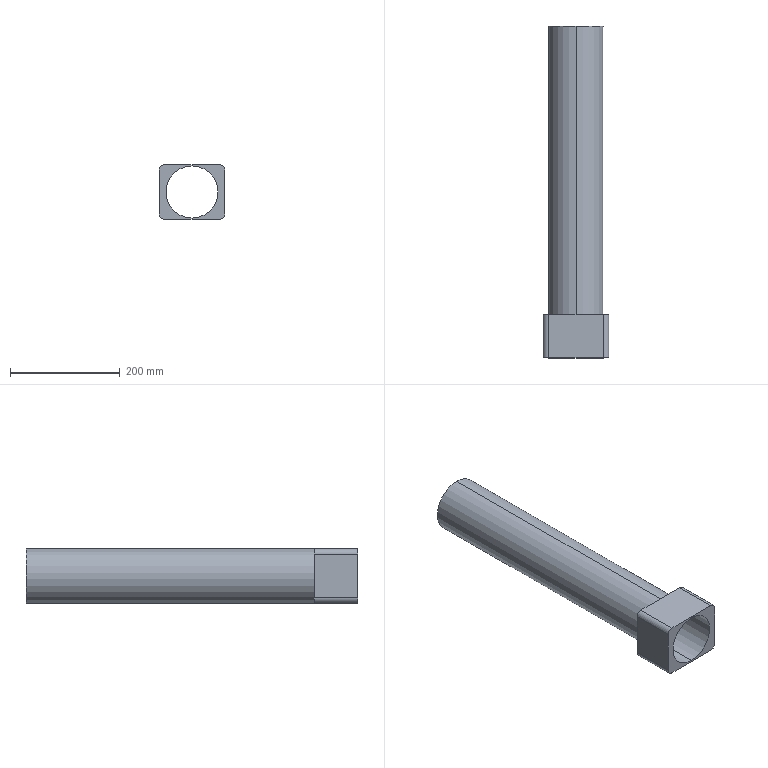Part | STEP file | Drain pipe 1 | 1 solid | 16 faces | box 120 x 605 x 100 mm | volume 788101 mm3 | cylinder 8 | plane 8 | commonest cylinder face diameters 20 x4 95 x2 100 x2
STEP:
#1=CARTESIAN_POINT('',(0.,0.,0.));
#2=DIRECTION('',(0.,0.,1.));
#3=DIRECTION('',(1.,0.,0.));
#4=AXIS2_PLACEMENT_3D('',#1,#2,#3);
#5=CARTESIAN_POINT('',(60.,605.,100.));
#6=VERTEX_POINT('',#5);
#7=CARTESIAN_POINT('',(60.,605.,0.));
#8=VERTEX_POINT('',#7);
#9=CARTESIAN_POINT('',(60.,605.,50.));
#10=DIRECTION('',(0.,1.,0.));
#11=DIRECTION('',(0.,0.,1.));
#12=AXIS2_PLACEMENT_3D('',#9,#10,#11);
#13=CIRCLE('',#12,50.);
#14=CARTESIAN_POINT('',(60.,605.,50.));
#15=DIRECTION('',(0.,-1.,0.));
#16=DIRECTION('',(0.,0.,-1.));
#17=AXIS2_PLACEMENT_3D('',#14,#15,#16);
#18=CYLINDRICAL_SURFACE('',#17,50.);
#19=CARTESIAN_POINT('',(3.142,0.));
#20=DIRECTION('',(-1.,0.));
#21=VECTOR('',#20,1.);
#22=LINE('',#19,#21);
#23=(GEOMETRIC_REPRESENTATION_CONTEXT(2)PARAMETRIC_REPRESENTATION_CONTEXT()REPRESENTATION_CONTEXT('',''));
#24=DEFINITIONAL_REPRESENTATION('',(#22),#23);
#25=PCURVE('',#18,#24);
#26=CARTESIAN_POINT('',(60.,605.,50.));
#27=DIRECTION('',(0.,1.,0.));
#28=DIRECTION('',(0.,0.,1.));
#29=AXIS2_PLACEMENT_3D('',#26,#27,#28);
#30=PLANE('',#29);
#31=CARTESIAN_POINT('',(0.,0.));
#32=DIRECTION('',(1.,0.));
#33=AXIS2_PLACEMENT_2D('',#31,#32);
#34=CIRCLE('',#33,50.);
#35=(GEOMETRIC_REPRESENTATION_CONTEXT(2)PARAMETRIC_REPRESENTATION_CONTEXT()REPRESENTATION_CONTEXT('',''));
#36=DEFINITIONAL_REPRESENTATION('',(#34),#35);
#37=PCURVE('',#30,#36);
#38=SURFACE_CURVE('',#13,(#25,#37),.PCURVE_S1.);
#39=EDGE_CURVE('',#6,#8,#38,.T.);
#40=ORIENTED_EDGE('',*,*,#39,.F.);
#41=CARTESIAN_POINT('',(60.,80.,100.));
#42=VERTEX_POINT('',#41);
#43=CARTESIAN_POINT('',(60.,605.,100.));
#44=DIRECTION('',(0.,-1.,0.));
#45=VECTOR('',#44,1.);
#46=LINE('',#43,#45);
#47=CARTESIAN_POINT('',(3.142,0.));
#48=DIRECTION('',(0.,1.));
#49=VECTOR('',#48,1.);
#50=LINE('',#47,#49);
#51=(GEOMETRIC_REPRESENTATION_CONTEXT(2)PARAMETRIC_REPRESENTATION_CONTEXT()REPRESENTATION_CONTEXT('',''));
#52=DEFINITIONAL_REPRESENTATION('',(#50),#51);
#53=PCURVE('',#18,#52);
#54=CARTESIAN_POINT('',(60.,605.,50.));
#55=DIRECTION('',(0.,-1.,0.));
#56=DIRECTION('',(0.,0.,-1.));
#57=AXIS2_PLACEMENT_3D('',#54,#55,#56);
#58=CYLINDRICAL_SURFACE('',#57,50.);
#59=CARTESIAN_POINT('',(3.142,0.));
#60=DIRECTION('',(0.,1.));
#61=VECTOR('',#60,1.);
#62=LINE('',#59,#61);
#63=(GEOMETRIC_REPRESENTATION_CONTEXT(2)PARAMETRIC_REPRESENTATION_CONTEXT()REPRESENTATION_CONTEXT('',''));
#64=DEFINITIONAL_REPRESENTATION('',(#62),#63);
#65=PCURVE('',#58,#64);
#66=SURFACE_CURVE('',#46,(#53,#65),.PCURVE_S1.);
#67=EDGE_CURVE('',#6,#42,#66,.T.);
#68=ORIENTED_EDGE('',*,*,#67,.T.);
#69=CARTESIAN_POINT('',(60.,80.,0.));
#70=VERTEX_POINT('',#69);
#71=CARTESIAN_POINT('',(60.,80.,50.));
#72=DIRECTION('',(0.,1.,0.));
#73=DIRECTION('',(0.,0.,1.));
#74=AXIS2_PLACEMENT_3D('',#71,#72,#73);
#75=CIRCLE('',#74,50.);
#76=CARTESIAN_POINT('',(3.142,525.));
#77=DIRECTION('',(-1.,0.));
#78=VECTOR('',#77,1.);
#79=LINE('',#76,#78);
#80=(GEOMETRIC_REPRESENTATION_CONTEXT(2)PARAMETRIC_REPRESENTATION_CONTEXT()REPRESENTATION_CONTEXT('',''));
#81=DEFINITIONAL_REPRESENTATION('',(#79),#80);
#82=PCURVE('',#18,#81);
#83=CARTESIAN_POINT('',(0.,80.,100.));
#84=DIRECTION('',(0.,1.,0.));
#85=DIRECTION('',(0.,0.,1.));
#86=AXIS2_PLACEMENT_3D('',#83,#84,#85);
#87=PLANE('',#86);
#88=CARTESIAN_POINT('',(-50.,60.));
#89=DIRECTION('',(1.,0.));
#90=AXIS2_PLACEMENT_2D('',#88,#89);
#91=CIRCLE('',#90,50.);
#92=(GEOMETRIC_REPRESENTATION_CONTEXT(2)PARAMETRIC_REPRESENTATION_CONTEXT()REPRESENTATION_CONTEXT('',''));
#93=DEFINITIONAL_REPRESENTATION('',(#91),#92);
#94=PCURVE('',#87,#93);
#95=SURFACE_CURVE('',#75,(#82,#94),.PCURVE_S1.);
#96=EDGE_CURVE('',#42,#70,#95,.T.);
#97=ORIENTED_EDGE('',*,*,#96,.T.);
#98=CARTESIAN_POINT('',(60.,605.,0.));
#99=DIRECTION('',(0.,-1.,0.));
#100=VECTOR('',#99,1.);
#101=LINE('',#98,#100);
#102=CARTESIAN_POINT('',(0.,0.));
#103=DIRECTION('',(0.,1.));
#104=VECTOR('',#103,1.);
#105=LINE('',#102,#104);
#106=(GEOMETRIC_REPRESENTATION_CONTEXT(2)PARAMETRIC_REPRESENTATION_CONTEXT()REPRESENTATION_CONTEXT('',''));
#107=DEFINITIONAL_REPRESENTATION('',(#105),#106);
#108=PCURVE('',#18,#107);
#109=CARTESIAN_POINT('',(6.283,0.));
#110=DIRECTION('',(0.,1.));
#111=VECTOR('',#110,1.);
#112=LINE('',#109,#111);
#113=(GEOMETRIC_REPRESENTATION_CONTEXT(2)PARAMETRIC_REPRESENTATION_CONTEXT()REPRESENTATION_CONTEXT('',''));
#114=DEFINITIONAL_REPRESENTATION('',(#112),#113);
#115=PCURVE('',#58,#114);
#116=SURFACE_CURVE('',#101,(#108,#115),.PCURVE_S1.);
#117=EDGE_CURVE('',#8,#70,#116,.T.);
#118=ORIENTED_EDGE('',*,*,#117,.F.);
#119=EDGE_LOOP('',(#40,#68,#97,#118));
#120=FACE_BOUND('',#119,.T.);
#121=ADVANCED_FACE('',(#120),#18,.T.);
#122=CARTESIAN_POINT('',(60.,605.,2.5));
#123=VERTEX_POINT('',#122);
#124=CARTESIAN_POINT('',(60.,0.,2.5));
#125=VERTEX_POINT('',#124);
#126=CARTESIAN_POINT('',(60.,605.,2.5));
#127=DIRECTION('',(0.,-1.,0.));
#128=VECTOR('',#127,1.);
#129=LINE('',#126,#128);
#130=CARTESIAN_POINT('',(60.,605.,50.));
#131=DIRECTION('',(0.,-1.,0.));
#132=DIRECTION('',(0.,0.,-1.));
#133=AXIS2_PLACEMENT_3D('',#130,#131,#132);
#134=CYLINDRICAL_SURFACE('',#133,47.5);
#135=CARTESIAN_POINT('',(6.283,0.));
#136=DIRECTION('',(0.,1.));
#137=VECTOR('',#136,1.);
#138=LINE('',#135,#137);
#139=(GEOMETRIC_REPRESENTATION_CONTEXT(2)PARAMETRIC_REPRESENTATION_CONTEXT()REPRESENTATION_CONTEXT('',''));
#140=DEFINITIONAL_REPRESENTATION('',(#138),#139);
#141=PCURVE('',#134,#140);
#142=CARTESIAN_POINT('',(60.,605.,50.));
#143=DIRECTION('',(0.,-1.,0.));
#144=DIRECTION('',(0.,0.,-1.));
#145=AXIS2_PLACEMENT_3D('',#142,#143,#144);
#146=CYLINDRICAL_SURFACE('',#145,47.5);
#147=CARTESIAN_POINT('',(0.,0.));
#148=DIRECTION('',(0.,1.));
#149=VECTOR('',#148,1.);
#150=LINE('',#147,#149);
#151=(GEOMETRIC_REPRESENTATION_CONTEXT(2)PARAMETRIC_REPRESENTATION_CONTEXT()REPRESENTATION_CONTEXT('',''));
#152=DEFINITIONAL_REPRESENTATION('',(#150),#151);
#153=PCURVE('',#146,#152);
#154=SURFACE_CURVE('',#129,(#141,#153),.PCURVE_S1.);
#155=EDGE_CURVE('',#123,#125,#154,.T.);
#156=ORIENTED_EDGE('',*,*,#155,.T.);
#157=CARTESIAN_POINT('',(60.,0.,97.5));
#158=VERTEX_POINT('',#157);
#159=CARTESIAN_POINT('',(60.,0.,50.));
#160=DIRECTION('',(0.,-1.,0.));
#161=DIRECTION('',(0.,0.,-1.));
#162=AXIS2_PLACEMENT_3D('',#159,#160,#161);
#163=CIRCLE('',#162,47.5);
#164=CARTESIAN_POINT('',(0.,605.));
#165=DIRECTION('',(1.,0.));
#166=VECTOR('',#165,1.);
#167=LINE('',#164,#166);
#168=(GEOMETRIC_REPRESENTATION_CONTEXT(2)PARAMETRIC_REPRESENTATION_CONTEXT()REPRESENTATION_CONTEXT('',''));
#169=DEFINITIONAL_REPRESENTATION('',(#167),#168);
#170=PCURVE('',#134,#169);
#171=CARTESIAN_POINT('',(0.,0.,100.));
#172=DIRECTION('',(0.,1.,0.));
#173=DIRECTION('',(0.,0.,1.));
#174=AXIS2_PLACEMENT_3D('',#171,#172,#173);
#175=PLANE('',#174);
#176=CARTESIAN_POINT('',(-97.5,60.));
#177=CARTESIAN_POINT('',(-97.5,142.272));
#178=CARTESIAN_POINT('',(-26.25,101.136));
#179=CARTESIAN_POINT('',(45.,60.));
#180=CARTESIAN_POINT('',(-26.25,18.864));
#181=CARTESIAN_POINT('',(-97.5,-22.272));
#182=CARTESIAN_POINT('',(-97.5,60.));
#183=(BOUNDED_CURVE()B_SPLINE_CURVE(2,(#176,#177,#178,#179,#180,#181,#182),.UNSPECIFIED.,.T.,.F.)B_SPLINE_CURVE_WITH_KNOTS((1,2,2,2,2,1),(-2.094,0.,2.094,4.189,6.283,8.378),.UNSPECIFIED.)CURVE()GEOMETRIC_REPRESENTATION_ITEM()RATIONAL_B_SPLINE_CURVE((1.,0.5,1.,0.5,1.,0.5,1.))REPRESENTATION_ITEM(''));
#184=(GEOMETRIC_REPRESENTATION_CONTEXT(2)PARAMETRIC_REPRESENTATION_CONTEXT()REPRESENTATION_CONTEXT('',''));
#185=DEFINITIONAL_REPRESENTATION('',(#183),#184);
#186=PCURVE('',#175,#185);
#187=SURFACE_CURVE('',#163,(#170,#186),.PCURVE_S1.);
#188=EDGE_CURVE('',#158,#125,#187,.T.);
#189=ORIENTED_EDGE('',*,*,#188,.F.);
#190=CARTESIAN_POINT('',(60.,605.,97.5));
#191=VERTEX_POINT('',#190);
#192=CARTESIAN_POINT('',(60.,605.,97.5));
#193=DIRECTION('',(0.,-1.,0.));
#194=VECTOR('',#193,1.);
#195=LINE('',#192,#194);
#196=CARTESIAN_POINT('',(3.142,0.));
#197=DIRECTION('',(0.,1.));
#198=VECTOR('',#197,1.);
#199=LINE('',#196,#198);
#200=(GEOMETRIC_REPRESENTATION_CONTEXT(2)PARAMETRIC_REPRESENTATION_CONTEXT()REPRESENTATION_CONTEXT('',''));
#201=DEFINITIONAL_REPRESENTATION('',(#199),#200);
#202=PCURVE('',#134,#201);
#203=CARTESIAN_POINT('',(3.142,0.));
#204=DIRECTION('',(0.,1.));
#205=VECTOR('',#204,1.);
#206=LINE('',#203,#205);
#207=(GEOMETRIC_REPRESENTATION_CONTEXT(2)PARAMETRIC_REPRESENTATION_CONTEXT()REPRESENTATION_CONTEXT('',''));
#208=DEFINITIONAL_REPRESENTATION('',(#206),#207);
#209=PCURVE('',#146,#208);
#210=SURFACE_CURVE('',#195,(#202,#209),.PCURVE_S1.);
#211=EDGE_CURVE('',#191,#158,#210,.T.);
#212=ORIENTED_EDGE('',*,*,#211,.F.);
#213=CARTESIAN_POINT('',(60.,605.,50.));
#214=DIRECTION('',(0.,1.,0.));
#215=DIRECTION('',(0.,0.,1.));
#216=AXIS2_PLACEMENT_3D('',#213,#214,#215);
#217=CIRCLE('',#216,47.5);
#218=CARTESIAN_POINT('',(9.425,0.));
#219=DIRECTION('',(-1.,0.));
#220=VECTOR('',#219,1.);
#221=LINE('',#218,#220);
#222=(GEOMETRIC_REPRESENTATION_CONTEXT(2)PARAMETRIC_REPRESENTATION_CONTEXT()REPRESENTATION_CONTEXT('',''));
#223=DEFINITIONAL_REPRESENTATION('',(#221),#222);
#224=PCURVE('',#134,#223);
#225=CARTESIAN_POINT('',(0.,0.));
#226=DIRECTION('',(1.,0.));
#227=AXIS2_PLACEMENT_2D('',#225,#226);
#228=CIRCLE('',#227,47.5);
#229=(GEOMETRIC_REPRESENTATION_CONTEXT(2)PARAMETRIC_REPRESENTATION_CONTEXT()REPRESENTATION_CONTEXT('',''));
#230=DEFINITIONAL_REPRESENTATION('',(#228),#229);
#231=PCURVE('',#30,#230);
#232=SURFACE_CURVE('',#217,(#224,#231),.PCURVE_S1.);
#233=EDGE_CURVE('',#123,#191,#232,.T.);
#234=ORIENTED_EDGE('',*,*,#233,.F.);
#235=EDGE_LOOP('',(#156,#189,#212,#234));
#236=FACE_BOUND('',#235,.F.);
#237=ADVANCED_FACE('',(#236),#134,.F.);
#238=CARTESIAN_POINT('',(110.,80.,100.));
#239=VERTEX_POINT('',#238);
#240=CARTESIAN_POINT('',(0.,80.,100.));
#241=DIRECTION('',(1.,0.,0.));
#242=VECTOR('',#241,1.);
#243=LINE('',#240,#242);
#244=CARTESIAN_POINT('',(0.,0.));
#245=DIRECTION('',(0.,1.));
#246=VECTOR('',#245,1.);
#247=LINE('',#244,#246);
#248=(GEOMETRIC_REPRESENTATION_CONTEXT(2)PARAMETRIC_REPRESENTATION_CONTEXT()REPRESENTATION_CONTEXT('',''));
#249=DEFINITIONAL_REPRESENTATION('',(#247),#248);
#250=PCURVE('',#87,#249);
#251=CARTESIAN_POINT('',(0.,80.,100.));
#252=DIRECTION('',(0.,0.,-1.));
#253=DIRECTION('',(-1.,0.,0.));
#254=AXIS2_PLACEMENT_3D('',#251,#252,#253);
#255=PLANE('',#254);
#256=CARTESIAN_POINT('',(0.,0.));
#257=DIRECTION('',(-1.,0.));
#258=VECTOR('',#257,1.);
#259=LINE('',#256,#258);
#260=(GEOMETRIC_REPRESENTATION_CONTEXT(2)PARAMETRIC_REPRESENTATION_CONTEXT()REPRESENTATION_CONTEXT('',''));
#261=DEFINITIONAL_REPRESENTATION('',(#259),#260);
#262=PCURVE('',#255,#261);
#263=SURFACE_CURVE('',#243,(#250,#262),.PCURVE_S1.);
#264=EDGE_CURVE('',#42,#239,#263,.T.);
#265=ORIENTED_EDGE('',*,*,#264,.T.);
#266=CARTESIAN_POINT('',(120.,80.,90.));
#267=VERTEX_POINT('',#266);
#268=CARTESIAN_POINT('',(110.,80.,90.));
#269=DIRECTION('',(0.,1.,0.));
#270=DIRECTION('',(0.,0.,1.));
#271=AXIS2_PLACEMENT_3D('',#268,#269,#270);
#272=CIRCLE('',#271,10.);
#273=CARTESIAN_POINT('',(-10.,110.));
#274=DIRECTION('',(1.,0.));
#275=AXIS2_PLACEMENT_2D('',#273,#274);
#276=CIRCLE('',#275,10.);
#277=(GEOMETRIC_REPRESENTATION_CONTEXT(2)PARAMETRIC_REPRESENTATION_CONTEXT()REPRESENTATION_CONTEXT('',''));
#278=DEFINITIONAL_REPRESENTATION('',(#276),#277);
#279=PCURVE('',#87,#278);
#280=CARTESIAN_POINT('',(110.,80.,90.));
#281=DIRECTION('',(0.,-1.,0.));
#282=DIRECTION('',(0.,0.,-1.));
#283=AXIS2_PLACEMENT_3D('',#280,#281,#282);
#284=CYLINDRICAL_SURFACE('',#283,10.);
#285=CARTESIAN_POINT('',(3.142,0.));
#286=DIRECTION('',(-1.,0.));
#287=VECTOR('',#286,1.);
#288=LINE('',#285,#287);
#289=(GEOMETRIC_REPRESENTATION_CONTEXT(2)PARAMETRIC_REPRESENTATION_CONTEXT()REPRESENTATION_CONTEXT('',''));
#290=DEFINITIONAL_REPRESENTATION('',(#288),#289);
#291=PCURVE('',#284,#290);
#292=SURFACE_CURVE('',#272,(#279,#291),.PCURVE_S1.);
#293=EDGE_CURVE('',#239,#267,#292,.T.);
#294=ORIENTED_EDGE('',*,*,#293,.T.);
#295=CARTESIAN_POINT('',(120.,80.,10.));
#296=VERTEX_POINT('',#295);
#297=CARTESIAN_POINT('',(120.,80.,0.));
#298=DIRECTION('',(0.,0.,-1.));
#299=VECTOR('',#298,1.);
#300=LINE('',#297,#299);
#301=CARTESIAN_POINT('',(-100.,120.));
#302=DIRECTION('',(-1.,0.));
#303=VECTOR('',#302,1.);
#304=LINE('',#301,#303);
#305=(GEOMETRIC_REPRESENTATION_CONTEXT(2)PARAMETRIC_REPRESENTATION_CONTEXT()REPRESENTATION_CONTEXT('',''));
#306=DEFINITIONAL_REPRESENTATION('',(#304),#305);
#307=PCURVE('',#87,#306);
#308=CARTESIAN_POINT('',(120.,80.,0.));
#309=DIRECTION('',(-1.,0.,0.));
#310=DIRECTION('',(0.,0.,1.));
#311=AXIS2_PLACEMENT_3D('',#308,#309,#310);
#312=PLANE('',#311);
#313=CARTESIAN_POINT('',(0.,0.));
#314=DIRECTION('',(-1.,0.));
#315=VECTOR('',#314,1.);
#316=LINE('',#313,#315);
#317=(GEOMETRIC_REPRESENTATION_CONTEXT(2)PARAMETRIC_REPRESENTATION_CONTEXT()REPRESENTATION_CONTEXT('',''));
#318=DEFINITIONAL_REPRESENTATION('',(#316),#317);
#319=PCURVE('',#312,#318);
#320=SURFACE_CURVE('',#300,(#307,#319),.PCURVE_S1.);
#321=EDGE_CURVE('',#267,#296,#320,.T.);
#322=ORIENTED_EDGE('',*,*,#321,.T.);
#323=CARTESIAN_POINT('',(110.,80.,0.));
#324=VERTEX_POINT('',#323);
#325=CARTESIAN_POINT('',(110.,80.,10.));
#326=DIRECTION('',(0.,1.,0.));
#327=DIRECTION('',(0.,0.,1.));
#328=AXIS2_PLACEMENT_3D('',#325,#326,#327);
#329=CIRCLE('',#328,10.);
#330=CARTESIAN_POINT('',(-90.,110.));
#331=DIRECTION('',(1.,0.));
#332=AXIS2_PLACEMENT_2D('',#330,#331);
#333=CIRCLE('',#332,10.);
#334=(GEOMETRIC_REPRESENTATION_CONTEXT(2)PARAMETRIC_REPRESENTATION_CONTEXT()REPRESENTATION_CONTEXT('',''));
#335=DEFINITIONAL_REPRESENTATION('',(#333),#334);
#336=PCURVE('',#87,#335);
#337=CARTESIAN_POINT('',(110.,80.,10.));
#338=DIRECTION('',(0.,-1.,0.));
#339=DIRECTION('',(0.,0.,-1.));
#340=AXIS2_PLACEMENT_3D('',#337,#338,#339);
#341=CYLINDRICAL_SURFACE('',#340,10.);
#342=CARTESIAN_POINT('',(3.142,0.));
#343=DIRECTION('',(-1.,0.));
#344=VECTOR('',#343,1.);
#345=LINE('',#342,#344);
#346=(GEOMETRIC_REPRESENTATION_CONTEXT(2)PARAMETRIC_REPRESENTATION_CONTEXT()REPRESENTATION_CONTEXT('',''));
#347=DEFINITIONAL_REPRESENTATION('',(#345),#346);
#348=PCURVE('',#341,#347);
#349=SURFACE_CURVE('',#329,(#336,#348),.PCURVE_S1.);
#350=EDGE_CURVE('',#296,#324,#349,.T.);
#351=ORIENTED_EDGE('',*,*,#350,.T.);
#352=CARTESIAN_POINT('',(0.,80.,0.));
#353=DIRECTION('',(-1.,0.,0.));
#354=VECTOR('',#353,1.);
#355=LINE('',#352,#354);
#356=CARTESIAN_POINT('',(-100.,0.));
#357=DIRECTION('',(0.,-1.));
#358=VECTOR('',#357,1.);
#359=LINE('',#356,#358);
#360=(GEOMETRIC_REPRESENTATION_CONTEXT(2)PARAMETRIC_REPRESENTATION_CONTEXT()REPRESENTATION_CONTEXT('',''));
#361=DEFINITIONAL_REPRESENTATION('',(#359),#360);
#362=PCURVE('',#87,#361);
#363=CARTESIAN_POINT('',(0.,80.,0.));
#364=DIRECTION('',(0.,0.,1.));
#365=DIRECTION('',(1.,0.,0.));
#366=AXIS2_PLACEMENT_3D('',#363,#364,#365);
#367=PLANE('',#366);
#368=CARTESIAN_POINT('',(0.,0.));
#369=DIRECTION('',(-1.,0.));
#370=VECTOR('',#369,1.);
#371=LINE('',#368,#370);
#372=(GEOMETRIC_REPRESENTATION_CONTEXT(2)PARAMETRIC_REPRESENTATION_CONTEXT()REPRESENTATION_CONTEXT('',''));
#373=DEFINITIONAL_REPRESENTATION('',(#371),#372);
#374=PCURVE('',#367,#373);
#375=SURFACE_CURVE('',#355,(#362,#374),.PCURVE_S1.);
#376=EDGE_CURVE('',#324,#70,#375,.T.);
#377=ORIENTED_EDGE('',*,*,#376,.T.);
#378=ORIENTED_EDGE('',*,*,#96,.F.);
#379=EDGE_LOOP('',(#265,#294,#322,#351,#377,#378));
#380=FACE_BOUND('',#379,.T.);
#381=ADVANCED_FACE('',(#380),#87,.T.);
#382=CARTESIAN_POINT('',(0.,80.,10.));
#383=VERTEX_POINT('',#382);
#384=CARTESIAN_POINT('',(0.,80.,90.));
#385=VERTEX_POINT('',#384);
#386=CARTESIAN_POINT('',(0.,80.,0.));
#387=DIRECTION('',(0.,0.,1.));
#388=VECTOR('',#387,1.);
#389=LINE('',#386,#388);
#390=CARTESIAN_POINT('',(0.,80.,0.));
#391=DIRECTION('',(1.,0.,0.));
#392=DIRECTION('',(0.,0.,-1.));
#393=AXIS2_PLACEMENT_3D('',#390,#391,#392);
#394=PLANE('',#393);
#395=CARTESIAN_POINT('',(0.,0.));
#396=DIRECTION('',(-1.,0.));
#397=VECTOR('',#396,1.);
#398=LINE('',#395,#397);
#399=(GEOMETRIC_REPRESENTATION_CONTEXT(2)PARAMETRIC_REPRESENTATION_CONTEXT()REPRESENTATION_CONTEXT('',''));
#400=DEFINITIONAL_REPRESENTATION('',(#398),#399);
#401=PCURVE('',#394,#400);
#402=CARTESIAN_POINT('',(0.,80.,100.));
#403=DIRECTION('',(0.,1.,0.));
#404=DIRECTION('',(0.,0.,1.));
#405=AXIS2_PLACEMENT_3D('',#402,#403,#404);
#406=PLANE('',#405);
#407=CARTESIAN_POINT('',(-100.,0.));
#408=DIRECTION('',(1.,0.));
#409=VECTOR('',#408,1.);
#410=LINE('',#407,#409);
#411=(GEOMETRIC_REPRESENTATION_CONTEXT(2)PARAMETRIC_REPRESENTATION_CONTEXT()REPRESENTATION_CONTEXT('',''));
#412=DEFINITIONAL_REPRESENTATION('',(#410),#411);
#413=PCURVE('',#406,#412);
#414=SURFACE_CURVE('',#389,(#401,#413),.PCURVE_S1.);
#415=EDGE_CURVE('',#383,#385,#414,.T.);
#416=ORIENTED_EDGE('',*,*,#415,.F.);
#417=CARTESIAN_POINT('',(0.,0.,10.));
#418=VERTEX_POINT('',#417);
#419=CARTESIAN_POINT('',(0.,80.,10.));
#420=DIRECTION('',(0.,-1.,0.));
#421=VECTOR('',#420,1.);
#422=LINE('',#419,#421);
#423=CARTESIAN_POINT('',(-10.,0.));
#424=DIRECTION('',(0.,-1.));
#425=VECTOR('',#424,1.);
#426=LINE('',#423,#425);
#427=(GEOMETRIC_REPRESENTATION_CONTEXT(2)PARAMETRIC_REPRESENTATION_CONTEXT()REPRESENTATION_CONTEXT('',''));
#428=DEFINITIONAL_REPRESENTATION('',(#426),#427);
#429=PCURVE('',#394,#428);
#430=CARTESIAN_POINT('',(10.,80.,10.));
#431=DIRECTION('',(0.,-1.,0.));
#432=DIRECTION('',(0.,0.,-1.));
#433=AXIS2_PLACEMENT_3D('',#430,#431,#432);
#434=CYLINDRICAL_SURFACE('',#433,10.);
#435=CARTESIAN_POINT('',(4.712,0.));
#436=DIRECTION('',(0.,1.));
#437=VECTOR('',#436,1.);
#438=LINE('',#435,#437);
#439=(GEOMETRIC_REPRESENTATION_CONTEXT(2)PARAMETRIC_REPRESENTATION_CONTEXT()REPRESENTATION_CONTEXT('',''));
#440=DEFINITIONAL_REPRESENTATION('',(#438),#439);
#441=PCURVE('',#434,#440);
#442=SURFACE_CURVE('',#422,(#429,#441),.PCURVE_S1.);
#443=EDGE_CURVE('',#383,#418,#442,.T.);
#444=ORIENTED_EDGE('',*,*,#443,.T.);
#445=CARTESIAN_POINT('',(0.,0.,90.));
#446=VERTEX_POINT('',#445);
#447=CARTESIAN_POINT('',(0.,0.,0.));
#448=DIRECTION('',(0.,0.,1.));
#449=VECTOR('',#448,1.);
#450=LINE('',#447,#449);
#451=CARTESIAN_POINT('',(0.,-80.));
#452=DIRECTION('',(-1.,0.));
#453=VECTOR('',#452,1.);
#454=LINE('',#451,#453);
#455=(GEOMETRIC_REPRESENTATION_CONTEXT(2)PARAMETRIC_REPRESENTATION_CONTEXT()REPRESENTATION_CONTEXT('',''));
#456=DEFINITIONAL_REPRESENTATION('',(#454),#455);
#457=PCURVE('',#394,#456);
#458=CARTESIAN_POINT('',(-100.,0.));
#459=DIRECTION('',(1.,0.));
#460=VECTOR('',#459,1.);
#461=LINE('',#458,#460);
#462=(GEOMETRIC_REPRESENTATION_CONTEXT(2)PARAMETRIC_REPRESENTATION_CONTEXT()REPRESENTATION_CONTEXT('',''));
#463=DEFINITIONAL_REPRESENTATION('',(#461),#462);
#464=PCURVE('',#175,#463);
#465=SURFACE_CURVE('',#450,(#457,#464),.PCURVE_S1.);
#466=EDGE_CURVE('',#418,#446,#465,.T.);
#467=ORIENTED_EDGE('',*,*,#466,.T.);
#468=CARTESIAN_POINT('',(0.,80.,90.));
#469=DIRECTION('',(0.,1.,0.));
#470=VECTOR('',#469,1.);
#471=LINE('',#468,#470);
#472=CARTESIAN_POINT('',(-90.,0.));
#473=DIRECTION('',(0.,1.));
#474=VECTOR('',#473,1.);
#475=LINE('',#472,#474);
#476=(GEOMETRIC_REPRESENTATION_CONTEXT(2)PARAMETRIC_REPRESENTATION_CONTEXT()REPRESENTATION_CONTEXT('',''));
#477=DEFINITIONAL_REPRESENTATION('',(#475),#476);
#478=PCURVE('',#394,#477);
#479=CARTESIAN_POINT('',(10.,80.,90.));
#480=DIRECTION('',(0.,-1.,0.));
#481=DIRECTION('',(0.,0.,-1.));
#482=AXIS2_PLACEMENT_3D('',#479,#480,#481);
#483=CYLINDRICAL_SURFACE('',#482,10.);
#484=CARTESIAN_POINT('',(4.712,0.));
#485=DIRECTION('',(0.,-1.));
#486=VECTOR('',#485,1.);
#487=LINE('',#484,#486);
#488=(GEOMETRIC_REPRESENTATION_CONTEXT(2)PARAMETRIC_REPRESENTATION_CONTEXT()REPRESENTATION_CONTEXT('',''));
#489=DEFINITIONAL_REPRESENTATION('',(#487),#488);
#490=PCURVE('',#483,#489);
#491=SURFACE_CURVE('',#471,(#478,#490),.PCURVE_S1.);
#492=EDGE_CURVE('',#446,#385,#491,.T.);
#493=ORIENTED_EDGE('',*,*,#492,.T.);
#494=EDGE_LOOP('',(#416,#444,#467,#493));
#495=FACE_BOUND('',#494,.T.);
#496=ADVANCED_FACE('',(#495),#394,.F.);
#497=CARTESIAN_POINT('',(10.,0.,100.));
#498=VERTEX_POINT('',#497);
#499=CARTESIAN_POINT('',(110.,0.,100.));
#500=VERTEX_POINT('',#499);
#501=CARTESIAN_POINT('',(0.,0.,100.));
#502=DIRECTION('',(1.,0.,0.));
#503=VECTOR('',#502,1.);
#504=LINE('',#501,#503);
#505=CARTESIAN_POINT('',(0.,-80.));
#506=DIRECTION('',(-1.,0.));
#507=VECTOR('',#506,1.);
#508=LINE('',#505,#507);
#509=(GEOMETRIC_REPRESENTATION_CONTEXT(2)PARAMETRIC_REPRESENTATION_CONTEXT()REPRESENTATION_CONTEXT('',''));
#510=DEFINITIONAL_REPRESENTATION('',(#508),#509);
#511=PCURVE('',#255,#510);
#512=CARTESIAN_POINT('',(0.,0.));
#513=DIRECTION('',(0.,1.));
#514=VECTOR('',#513,1.);
#515=LINE('',#512,#514);
#516=(GEOMETRIC_REPRESENTATION_CONTEXT(2)PARAMETRIC_REPRESENTATION_CONTEXT()REPRESENTATION_CONTEXT('',''));
#517=DEFINITIONAL_REPRESENTATION('',(#515),#516);
#518=PCURVE('',#175,#517);
#519=SURFACE_CURVE('',#504,(#511,#518),.PCURVE_S1.);
#520=EDGE_CURVE('',#498,#500,#519,.T.);
#521=ORIENTED_EDGE('',*,*,#520,.T.);
#522=CARTESIAN_POINT('',(110.,80.,100.));
#523=DIRECTION('',(0.,1.,0.));
#524=VECTOR('',#523,1.);
#525=LINE('',#522,#524);
#526=CARTESIAN_POINT('',(-110.,0.));
#527=DIRECTION('',(0.,1.));
#528=VECTOR('',#527,1.);
#529=LINE('',#526,#528);
#530=(GEOMETRIC_REPRESENTATION_CONTEXT(2)PARAMETRIC_REPRESENTATION_CONTEXT()REPRESENTATION_CONTEXT('',''));
#531=DEFINITIONAL_REPRESENTATION('',(#529),#530);
#532=PCURVE('',#255,#531);
#533=CARTESIAN_POINT('',(3.142,0.));
#534=DIRECTION('',(0.,-1.));
#535=VECTOR('',#534,1.);
#536=LINE('',#533,#535);
#537=(GEOMETRIC_REPRESENTATION_CONTEXT(2)PARAMETRIC_REPRESENTATION_CONTEXT()REPRESENTATION_CONTEXT('',''));
#538=DEFINITIONAL_REPRESENTATION('',(#536),#537);
#539=PCURVE('',#284,#538);
#540=SURFACE_CURVE('',#525,(#532,#539),.PCURVE_S1.);
#541=EDGE_CURVE('',#500,#239,#540,.T.);
#542=ORIENTED_EDGE('',*,*,#541,.T.);
#543=ORIENTED_EDGE('',*,*,#264,.F.);
#544=CARTESIAN_POINT('',(10.,80.,100.));
#545=VERTEX_POINT('',#544);
#546=CARTESIAN_POINT('',(0.,80.,100.));
#547=DIRECTION('',(1.,0.,0.));
#548=VECTOR('',#547,1.);
#549=LINE('',#546,#548);
#550=CARTESIAN_POINT('',(0.,0.));
#551=DIRECTION('',(-1.,0.));
#552=VECTOR('',#551,1.);
#553=LINE('',#550,#552);
#554=(GEOMETRIC_REPRESENTATION_CONTEXT(2)PARAMETRIC_REPRESENTATION_CONTEXT()REPRESENTATION_CONTEXT('',''));
#555=DEFINITIONAL_REPRESENTATION('',(#553),#554);
#556=PCURVE('',#255,#555);
#557=CARTESIAN_POINT('',(0.,0.));
#558=DIRECTION('',(0.,1.));
#559=VECTOR('',#558,1.);
#560=LINE('',#557,#559);
#561=(GEOMETRIC_REPRESENTATION_CONTEXT(2)PARAMETRIC_REPRESENTATION_CONTEXT()REPRESENTATION_CONTEXT('',''));
#562=DEFINITIONAL_REPRESENTATION('',(#560),#561);
#563=PCURVE('',#406,#562);
#564=SURFACE_CURVE('',#549,(#556,#563),.PCURVE_S1.);
#565=EDGE_CURVE('',#545,#42,#564,.T.);
#566=ORIENTED_EDGE('',*,*,#565,.F.);
#567=CARTESIAN_POINT('',(10.,80.,100.));
#568=DIRECTION('',(0.,-1.,0.));
#569=VECTOR('',#568,1.);
#570=LINE('',#567,#569);
#571=CARTESIAN_POINT('',(-10.,0.));
#572=DIRECTION('',(0.,-1.));
#573=VECTOR('',#572,1.);
#574=LINE('',#571,#573);
#575=(GEOMETRIC_REPRESENTATION_CONTEXT(2)PARAMETRIC_REPRESENTATION_CONTEXT()REPRESENTATION_CONTEXT('',''));
#576=DEFINITIONAL_REPRESENTATION('',(#574),#575);
#577=PCURVE('',#255,#576);
#578=CARTESIAN_POINT('',(3.142,0.));
#579=DIRECTION('',(0.,1.));
#580=VECTOR('',#579,1.);
#581=LINE('',#578,#580);
#582=(GEOMETRIC_REPRESENTATION_CONTEXT(2)PARAMETRIC_REPRESENTATION_CONTEXT()REPRESENTATION_CONTEXT('',''));
#583=DEFINITIONAL_REPRESENTATION('',(#581),#582);
#584=PCURVE('',#483,#583);
#585=SURFACE_CURVE('',#570,(#577,#584),.PCURVE_S1.);
#586=EDGE_CURVE('',#545,#498,#585,.T.);
#587=ORIENTED_EDGE('',*,*,#586,.T.);
#588=EDGE_LOOP('',(#521,#542,#543,#566,#587));
#589=FACE_BOUND('',#588,.T.);
#590=ADVANCED_FACE('',(#589),#255,.F.);
#591=ORIENTED_EDGE('',*,*,#321,.F.);
#592=CARTESIAN_POINT('',(120.,0.,90.));
#593=VERTEX_POINT('',#592);
#594=CARTESIAN_POINT('',(120.,80.,90.));
#595=DIRECTION('',(0.,-1.,0.));
#596=VECTOR('',#595,1.);
#597=LINE('',#594,#596);
#598=CARTESIAN_POINT('',(90.,0.));
#599=DIRECTION('',(0.,-1.));
#600=VECTOR('',#599,1.);
#601=LINE('',#598,#600);
#602=(GEOMETRIC_REPRESENTATION_CONTEXT(2)PARAMETRIC_REPRESENTATION_CONTEXT()REPRESENTATION_CONTEXT('',''));
#603=DEFINITIONAL_REPRESENTATION('',(#601),#602);
#604=PCURVE('',#312,#603);
#605=CARTESIAN_POINT('',(1.571,0.));
#606=DIRECTION('',(0.,1.));
#607=VECTOR('',#606,1.);
#608=LINE('',#605,#607);
#609=(GEOMETRIC_REPRESENTATION_CONTEXT(2)PARAMETRIC_REPRESENTATION_CONTEXT()REPRESENTATION_CONTEXT('',''));
#610=DEFINITIONAL_REPRESENTATION('',(#608),#609);
#611=PCURVE('',#284,#610);
#612=SURFACE_CURVE('',#597,(#604,#611),.PCURVE_S1.);
#613=EDGE_CURVE('',#267,#593,#612,.T.);
#614=ORIENTED_EDGE('',*,*,#613,.T.);
#615=CARTESIAN_POINT('',(120.,0.,10.));
#616=VERTEX_POINT('',#615);
#617=CARTESIAN_POINT('',(120.,0.,0.));
#618=DIRECTION('',(0.,0.,-1.));
#619=VECTOR('',#618,1.);
#620=LINE('',#617,#619);
#621=CARTESIAN_POINT('',(0.,-80.));
#622=DIRECTION('',(-1.,0.));
#623=VECTOR('',#622,1.);
#624=LINE('',#621,#623);
#625=(GEOMETRIC_REPRESENTATION_CONTEXT(2)PARAMETRIC_REPRESENTATION_CONTEXT()REPRESENTATION_CONTEXT('',''));
#626=DEFINITIONAL_REPRESENTATION('',(#624),#625);
#627=PCURVE('',#312,#626);
#628=CARTESIAN_POINT('',(-100.,120.));
#629=DIRECTION('',(-1.,0.));
#630=VECTOR('',#629,1.);
#631=LINE('',#628,#630);
#632=(GEOMETRIC_REPRESENTATION_CONTEXT(2)PARAMETRIC_REPRESENTATION_CONTEXT()REPRESENTATION_CONTEXT('',''));
#633=DEFINITIONAL_REPRESENTATION('',(#631),#632);
#634=PCURVE('',#175,#633);
#635=SURFACE_CURVE('',#620,(#627,#634),.PCURVE_S1.);
#636=EDGE_CURVE('',#593,#616,#635,.T.);
#637=ORIENTED_EDGE('',*,*,#636,.T.);
#638=CARTESIAN_POINT('',(120.,80.,10.));
#639=DIRECTION('',(0.,1.,0.));
#640=VECTOR('',#639,1.);
#641=LINE('',#638,#640);
#642=CARTESIAN_POINT('',(10.,0.));
#643=DIRECTION('',(0.,1.));
#644=VECTOR('',#643,1.);
#645=LINE('',#642,#644);
#646=(GEOMETRIC_REPRESENTATION_CONTEXT(2)PARAMETRIC_REPRESENTATION_CONTEXT()REPRESENTATION_CONTEXT('',''));
#647=DEFINITIONAL_REPRESENTATION('',(#645),#646);
#648=PCURVE('',#312,#647);
#649=CARTESIAN_POINT('',(1.571,0.));
#650=DIRECTION('',(0.,-1.));
#651=VECTOR('',#650,1.);
#652=LINE('',#649,#651);
#653=(GEOMETRIC_REPRESENTATION_CONTEXT(2)PARAMETRIC_REPRESENTATION_CONTEXT()REPRESENTATION_CONTEXT('',''));
#654=DEFINITIONAL_REPRESENTATION('',(#652),#653);
#655=PCURVE('',#341,#654);
#656=SURFACE_CURVE('',#641,(#648,#655),.PCURVE_S1.);
#657=EDGE_CURVE('',#616,#296,#656,.T.);
#658=ORIENTED_EDGE('',*,*,#657,.T.);
#659=EDGE_LOOP('',(#591,#614,#637,#658));
#660=FACE_BOUND('',#659,.T.);
#661=ADVANCED_FACE('',(#660),#312,.F.);
#662=ORIENTED_EDGE('',*,*,#376,.F.);
#663=CARTESIAN_POINT('',(110.,0.,0.));
#664=VERTEX_POINT('',#663);
#665=CARTESIAN_POINT('',(110.,80.,0.));
#666=DIRECTION('',(0.,-1.,0.));
#667=VECTOR('',#666,1.);
#668=LINE('',#665,#667);
#669=CARTESIAN_POINT('',(110.,0.));
#670=DIRECTION('',(0.,-1.));
#671=VECTOR('',#670,1.);
#672=LINE('',#669,#671);
#673=(GEOMETRIC_REPRESENTATION_CONTEXT(2)PARAMETRIC_REPRESENTATION_CONTEXT()REPRESENTATION_CONTEXT('',''));
#674=DEFINITIONAL_REPRESENTATION('',(#672),#673);
#675=PCURVE('',#367,#674);
#676=CARTESIAN_POINT('',(0.,0.));
#677=DIRECTION('',(0.,1.));
#678=VECTOR('',#677,1.);
#679=LINE('',#676,#678);
#680=(GEOMETRIC_REPRESENTATION_CONTEXT(2)PARAMETRIC_REPRESENTATION_CONTEXT()REPRESENTATION_CONTEXT('',''));
#681=DEFINITIONAL_REPRESENTATION('',(#679),#680);
#682=PCURVE('',#341,#681);
#683=SURFACE_CURVE('',#668,(#675,#682),.PCURVE_S1.);
#684=EDGE_CURVE('',#324,#664,#683,.T.);
#685=ORIENTED_EDGE('',*,*,#684,.T.);
#686=CARTESIAN_POINT('',(10.,0.,0.));
#687=VERTEX_POINT('',#686);
#688=CARTESIAN_POINT('',(0.,0.,0.));
#689=DIRECTION('',(-1.,0.,0.));
#690=VECTOR('',#689,1.);
#691=LINE('',#688,#690);
#692=CARTESIAN_POINT('',(0.,-80.));
#693=DIRECTION('',(-1.,0.));
#694=VECTOR('',#693,1.);
#695=LINE('',#692,#694);
#696=(GEOMETRIC_REPRESENTATION_CONTEXT(2)PARAMETRIC_REPRESENTATION_CONTEXT()REPRESENTATION_CONTEXT('',''));
#697=DEFINITIONAL_REPRESENTATION('',(#695),#696);
#698=PCURVE('',#367,#697);
#699=CARTESIAN_POINT('',(-100.,0.));
#700=DIRECTION('',(0.,-1.));
#701=VECTOR('',#700,1.);
#702=LINE('',#699,#701);
#703=(GEOMETRIC_REPRESENTATION_CONTEXT(2)PARAMETRIC_REPRESENTATION_CONTEXT()REPRESENTATION_CONTEXT('',''));
#704=DEFINITIONAL_REPRESENTATION('',(#702),#703);
#705=PCURVE('',#175,#704);
#706=SURFACE_CURVE('',#691,(#698,#705),.PCURVE_S1.);
#707=EDGE_CURVE('',#664,#687,#706,.T.);
#708=ORIENTED_EDGE('',*,*,#707,.T.);
#709=CARTESIAN_POINT('',(10.,80.,0.));
#710=VERTEX_POINT('',#709);
#711=CARTESIAN_POINT('',(10.,80.,0.));
#712=DIRECTION('',(0.,1.,0.));
#713=VECTOR('',#712,1.);
#714=LINE('',#711,#713);
#715=CARTESIAN_POINT('',(10.,0.));
#716=DIRECTION('',(0.,1.));
#717=VECTOR('',#716,1.);
#718=LINE('',#715,#717);
#719=(GEOMETRIC_REPRESENTATION_CONTEXT(2)PARAMETRIC_REPRESENTATION_CONTEXT()REPRESENTATION_CONTEXT('',''));
#720=DEFINITIONAL_REPRESENTATION('',(#718),#719);
#721=PCURVE('',#367,#720);
#722=CARTESIAN_POINT('',(6.283,0.));
#723=DIRECTION('',(0.,-1.));
#724=VECTOR('',#723,1.);
#725=LINE('',#722,#724);
#726=(GEOMETRIC_REPRESENTATION_CONTEXT(2)PARAMETRIC_REPRESENTATION_CONTEXT()REPRESENTATION_CONTEXT('',''));
#727=DEFINITIONAL_REPRESENTATION('',(#725),#726);
#728=PCURVE('',#434,#727);
#729=SURFACE_CURVE('',#714,(#721,#728),.PCURVE_S1.);
#730=EDGE_CURVE('',#687,#710,#729,.T.);
#731=ORIENTED_EDGE('',*,*,#730,.T.);
#732=CARTESIAN_POINT('',(0.,80.,0.));
#733=DIRECTION('',(-1.,0.,0.));
#734=VECTOR('',#733,1.);
#735=LINE('',#732,#734);
#736=CARTESIAN_POINT('',(0.,0.));
#737=DIRECTION('',(-1.,0.));
#738=VECTOR('',#737,1.);
#739=LINE('',#736,#738);
#740=(GEOMETRIC_REPRESENTATION_CONTEXT(2)PARAMETRIC_REPRESENTATION_CONTEXT()REPRESENTATION_CONTEXT('',''));
#741=DEFINITIONAL_REPRESENTATION('',(#739),#740);
#742=PCURVE('',#367,#741);
#743=CARTESIAN_POINT('',(-100.,0.));
#744=DIRECTION('',(0.,-1.));
#745=VECTOR('',#744,1.);
#746=LINE('',#743,#745);
#747=(GEOMETRIC_REPRESENTATION_CONTEXT(2)PARAMETRIC_REPRESENTATION_CONTEXT()REPRESENTATION_CONTEXT('',''));
#748=DEFINITIONAL_REPRESENTATION('',(#746),#747);
#749=PCURVE('',#406,#748);
#750=SURFACE_CURVE('',#735,(#742,#749),.PCURVE_S1.);
#751=EDGE_CURVE('',#70,#710,#750,.T.);
#752=ORIENTED_EDGE('',*,*,#751,.F.);
#753=EDGE_LOOP('',(#662,#685,#708,#731,#752));
#754=FACE_BOUND('',#753,.T.);
#755=ADVANCED_FACE('',(#754),#367,.F.);
#756=ORIENTED_EDGE('',*,*,#751,.T.);
#757=CARTESIAN_POINT('',(10.,80.,10.));
#758=DIRECTION('',(0.,1.,0.));
#759=DIRECTION('',(0.,0.,1.));
#760=AXIS2_PLACEMENT_3D('',#757,#758,#759);
#761=CIRCLE('',#760,10.);
#762=CARTESIAN_POINT('',(-90.,10.));
#763=DIRECTION('',(1.,0.));
#764=AXIS2_PLACEMENT_2D('',#762,#763);
#765=CIRCLE('',#764,10.);
#766=(GEOMETRIC_REPRESENTATION_CONTEXT(2)PARAMETRIC_REPRESENTATION_CONTEXT()REPRESENTATION_CONTEXT('',''));
#767=DEFINITIONAL_REPRESENTATION('',(#765),#766);
#768=PCURVE('',#406,#767);
#769=CARTESIAN_POINT('',(9.425,0.));
#770=DIRECTION('',(-1.,0.));
#771=VECTOR('',#770,1.);
#772=LINE('',#769,#771);
#773=(GEOMETRIC_REPRESENTATION_CONTEXT(2)PARAMETRIC_REPRESENTATION_CONTEXT()REPRESENTATION_CONTEXT('',''));
#774=DEFINITIONAL_REPRESENTATION('',(#772),#773);
#775=PCURVE('',#434,#774);
#776=SURFACE_CURVE('',#761,(#768,#775),.PCURVE_S1.);
#777=EDGE_CURVE('',#710,#383,#776,.T.);
#778=ORIENTED_EDGE('',*,*,#777,.T.);
#779=ORIENTED_EDGE('',*,*,#415,.T.);
#780=CARTESIAN_POINT('',(10.,80.,90.));
#781=DIRECTION('',(0.,1.,0.));
#782=DIRECTION('',(0.,0.,1.));
#783=AXIS2_PLACEMENT_3D('',#780,#781,#782);
#784=CIRCLE('',#783,10.);
#785=CARTESIAN_POINT('',(-10.,10.));
#786=DIRECTION('',(1.,0.));
#787=AXIS2_PLACEMENT_2D('',#785,#786);
#788=CIRCLE('',#787,10.);
#789=(GEOMETRIC_REPRESENTATION_CONTEXT(2)PARAMETRIC_REPRESENTATION_CONTEXT()REPRESENTATION_CONTEXT('',''));
#790=DEFINITIONAL_REPRESENTATION('',(#788),#789);
#791=PCURVE('',#406,#790);
#792=CARTESIAN_POINT('',(9.425,0.));
#793=DIRECTION('',(-1.,0.));
#794=VECTOR('',#793,1.);
#795=LINE('',#792,#794);
#796=(GEOMETRIC_REPRESENTATION_CONTEXT(2)PARAMETRIC_REPRESENTATION_CONTEXT()REPRESENTATION_CONTEXT('',''));
#797=DEFINITIONAL_REPRESENTATION('',(#795),#796);
#798=PCURVE('',#483,#797);
#799=SURFACE_CURVE('',#784,(#791,#798),.PCURVE_S1.);
#800=EDGE_CURVE('',#385,#545,#799,.T.);
#801=ORIENTED_EDGE('',*,*,#800,.T.);
#802=ORIENTED_EDGE('',*,*,#565,.T.);
#803=CARTESIAN_POINT('',(60.,80.,50.));
#804=DIRECTION('',(0.,1.,0.));
#805=DIRECTION('',(0.,0.,1.));
#806=AXIS2_PLACEMENT_3D('',#803,#804,#805);
#807=CIRCLE('',#806,50.);
#808=CARTESIAN_POINT('',(-50.,60.));
#809=DIRECTION('',(1.,0.));
#810=AXIS2_PLACEMENT_2D('',#808,#809);
#811=CIRCLE('',#810,50.);
#812=(GEOMETRIC_REPRESENTATION_CONTEXT(2)PARAMETRIC_REPRESENTATION_CONTEXT()REPRESENTATION_CONTEXT('',''));
#813=DEFINITIONAL_REPRESENTATION('',(#811),#812);
#814=PCURVE('',#406,#813);
#815=CARTESIAN_POINT('',(9.425,525.));
#816=DIRECTION('',(-1.,0.));
#817=VECTOR('',#816,1.);
#818=LINE('',#815,#817);
#819=(GEOMETRIC_REPRESENTATION_CONTEXT(2)PARAMETRIC_REPRESENTATION_CONTEXT()REPRESENTATION_CONTEXT('',''));
#820=DEFINITIONAL_REPRESENTATION('',(#818),#819);
#821=PCURVE('',#58,#820);
#822=SURFACE_CURVE('',#807,(#814,#821),.PCURVE_S1.);
#823=EDGE_CURVE('',#70,#42,#822,.T.);
#824=ORIENTED_EDGE('',*,*,#823,.F.);
#825=EDGE_LOOP('',(#756,#778,#779,#801,#802,#824));
#826=FACE_BOUND('',#825,.T.);
#827=ADVANCED_FACE('',(#826),#406,.T.);
#828=CARTESIAN_POINT('',(60.,0.,50.));
#829=DIRECTION('',(0.,-1.,0.));
#830=DIRECTION('',(0.,0.,-1.));
#831=AXIS2_PLACEMENT_3D('',#828,#829,#830);
#832=CIRCLE('',#831,47.5);
#833=CARTESIAN_POINT('',(-97.5,60.));
#834=CARTESIAN_POINT('',(-97.5,142.272));
#835=CARTESIAN_POINT('',(-26.25,101.136));
#836=CARTESIAN_POINT('',(45.,60.));
#837=CARTESIAN_POINT('',(-26.25,18.864));
#838=CARTESIAN_POINT('',(-97.5,-22.272));
#839=CARTESIAN_POINT('',(-97.5,60.));
#840=(BOUNDED_CURVE()B_SPLINE_CURVE(2,(#833,#834,#835,#836,#837,#838,#839),.UNSPECIFIED.,.T.,.F.)B_SPLINE_CURVE_WITH_KNOTS((1,2,2,2,2,1),(-2.094,0.,2.094,4.189,6.283,8.378),.UNSPECIFIED.)CURVE()GEOMETRIC_REPRESENTATION_ITEM()RATIONAL_B_SPLINE_CURVE((1.,0.5,1.,0.5,1.,0.5,1.))REPRESENTATION_ITEM(''));
#841=(GEOMETRIC_REPRESENTATION_CONTEXT(2)PARAMETRIC_REPRESENTATION_CONTEXT()REPRESENTATION_CONTEXT('',''));
#842=DEFINITIONAL_REPRESENTATION('',(#840),#841);
#843=PCURVE('',#175,#842);
#844=CARTESIAN_POINT('',(0.,605.));
#845=DIRECTION('',(1.,0.));
#846=VECTOR('',#845,1.);
#847=LINE('',#844,#846);
#848=(GEOMETRIC_REPRESENTATION_CONTEXT(2)PARAMETRIC_REPRESENTATION_CONTEXT()REPRESENTATION_CONTEXT('',''));
#849=DEFINITIONAL_REPRESENTATION('',(#847),#848);
#850=PCURVE('',#146,#849);
#851=SURFACE_CURVE('',#832,(#843,#850),.PCURVE_S1.);
#852=EDGE_CURVE('',#125,#158,#851,.T.);
#853=ORIENTED_EDGE('',*,*,#852,.F.);
#854=ORIENTED_EDGE('',*,*,#188,.F.);
#855=EDGE_LOOP('',(#853,#854));
#856=FACE_BOUND('',#855,.T.);
#857=ORIENTED_EDGE('',*,*,#636,.F.);
#858=CARTESIAN_POINT('',(110.,0.,90.));
#859=DIRECTION('',(0.,-1.,0.));
#860=DIRECTION('',(0.,0.,1.));
#861=AXIS2_PLACEMENT_3D('',#858,#859,#860);
#862=CIRCLE('',#861,10.);
#863=CARTESIAN_POINT('',(0.,110.));
#864=CARTESIAN_POINT('',(0.,92.679));
#865=CARTESIAN_POINT('',(-15.,101.34));
#866=CARTESIAN_POINT('',(-30.,110.));
#867=CARTESIAN_POINT('',(-15.,118.66));
#868=CARTESIAN_POINT('',(0.,127.321));
#869=CARTESIAN_POINT('',(0.,110.));
#870=(BOUNDED_CURVE()B_SPLINE_CURVE(2,(#863,#864,#865,#866,#867,#868,#869),.UNSPECIFIED.,.T.,.F.)B_SPLINE_CURVE_WITH_KNOTS((1,2,2,2,2,1),(-2.094,0.,2.094,4.189,6.283,8.378),.UNSPECIFIED.)CURVE()GEOMETRIC_REPRESENTATION_ITEM()RATIONAL_B_SPLINE_CURVE((1.,0.5,1.,0.5,1.,0.5,1.))REPRESENTATION_ITEM(''));
#871=(GEOMETRIC_REPRESENTATION_CONTEXT(2)PARAMETRIC_REPRESENTATION_CONTEXT()REPRESENTATION_CONTEXT('',''));
#872=DEFINITIONAL_REPRESENTATION('',(#870),#871);
#873=PCURVE('',#175,#872);
#874=CARTESIAN_POINT('',(-3.142,80.));
#875=DIRECTION('',(1.,0.));
#876=VECTOR('',#875,1.);
#877=LINE('',#874,#876);
#878=(GEOMETRIC_REPRESENTATION_CONTEXT(2)PARAMETRIC_REPRESENTATION_CONTEXT()REPRESENTATION_CONTEXT('',''));
#879=DEFINITIONAL_REPRESENTATION('',(#877),#878);
#880=PCURVE('',#284,#879);
#881=SURFACE_CURVE('',#862,(#873,#880),.PCURVE_S1.);
#882=EDGE_CURVE('',#593,#500,#881,.T.);
#883=ORIENTED_EDGE('',*,*,#882,.T.);
#884=ORIENTED_EDGE('',*,*,#520,.F.);
#885=CARTESIAN_POINT('',(10.,0.,90.));
#886=DIRECTION('',(0.,-1.,0.));
#887=DIRECTION('',(0.,0.,1.));
#888=AXIS2_PLACEMENT_3D('',#885,#886,#887);
#889=CIRCLE('',#888,10.);
#890=CARTESIAN_POINT('',(0.,10.));
#891=CARTESIAN_POINT('',(0.,-7.321));
#892=CARTESIAN_POINT('',(-15.,1.34));
#893=CARTESIAN_POINT('',(-30.,10.));
#894=CARTESIAN_POINT('',(-15.,18.66));
#895=CARTESIAN_POINT('',(0.,27.321));
#896=CARTESIAN_POINT('',(0.,10.));
#897=(BOUNDED_CURVE()B_SPLINE_CURVE(2,(#890,#891,#892,#893,#894,#895,#896),.UNSPECIFIED.,.T.,.F.)B_SPLINE_CURVE_WITH_KNOTS((1,2,2,2,2,1),(-2.094,0.,2.094,4.189,6.283,8.378),.UNSPECIFIED.)CURVE()GEOMETRIC_REPRESENTATION_ITEM()RATIONAL_B_SPLINE_CURVE((1.,0.5,1.,0.5,1.,0.5,1.))REPRESENTATION_ITEM(''));
#898=(GEOMETRIC_REPRESENTATION_CONTEXT(2)PARAMETRIC_REPRESENTATION_CONTEXT()REPRESENTATION_CONTEXT('',''));
#899=DEFINITIONAL_REPRESENTATION('',(#897),#898);
#900=PCURVE('',#175,#899);
#901=CARTESIAN_POINT('',(3.142,80.));
#902=DIRECTION('',(1.,0.));
#903=VECTOR('',#902,1.);
#904=LINE('',#901,#903);
#905=(GEOMETRIC_REPRESENTATION_CONTEXT(2)PARAMETRIC_REPRESENTATION_CONTEXT()REPRESENTATION_CONTEXT('',''));
#906=DEFINITIONAL_REPRESENTATION('',(#904),#905);
#907=PCURVE('',#483,#906);
#908=SURFACE_CURVE('',#889,(#900,#907),.PCURVE_S1.);
#909=EDGE_CURVE('',#498,#446,#908,.T.);
#910=ORIENTED_EDGE('',*,*,#909,.T.);
#911=ORIENTED_EDGE('',*,*,#466,.F.);
#912=CARTESIAN_POINT('',(10.,0.,10.));
#913=DIRECTION('',(0.,-1.,0.));
#914=DIRECTION('',(0.,0.,1.));
#915=AXIS2_PLACEMENT_3D('',#912,#913,#914);
#916=CIRCLE('',#915,10.);
#917=CARTESIAN_POINT('',(-80.,10.));
#918=CARTESIAN_POINT('',(-80.,-7.321));
#919=CARTESIAN_POINT('',(-95.,1.34));
#920=CARTESIAN_POINT('',(-110.,10.));
#921=CARTESIAN_POINT('',(-95.,18.66));
#922=CARTESIAN_POINT('',(-80.,27.321));
#923=CARTESIAN_POINT('',(-80.,10.));
#924=(BOUNDED_CURVE()B_SPLINE_CURVE(2,(#917,#918,#919,#920,#921,#922,#923),.UNSPECIFIED.,.T.,.F.)B_SPLINE_CURVE_WITH_KNOTS((1,2,2,2,2,1),(-2.094,0.,2.094,4.189,6.283,8.378),.UNSPECIFIED.)CURVE()GEOMETRIC_REPRESENTATION_ITEM()RATIONAL_B_SPLINE_CURVE((1.,0.5,1.,0.5,1.,0.5,1.))REPRESENTATION_ITEM(''));
#925=(GEOMETRIC_REPRESENTATION_CONTEXT(2)PARAMETRIC_REPRESENTATION_CONTEXT()REPRESENTATION_CONTEXT('',''));
#926=DEFINITIONAL_REPRESENTATION('',(#924),#925);
#927=PCURVE('',#175,#926);
#928=CARTESIAN_POINT('',(3.142,80.));
#929=DIRECTION('',(1.,0.));
#930=VECTOR('',#929,1.);
#931=LINE('',#928,#930);
#932=(GEOMETRIC_REPRESENTATION_CONTEXT(2)PARAMETRIC_REPRESENTATION_CONTEXT()REPRESENTATION_CONTEXT('',''));
#933=DEFINITIONAL_REPRESENTATION('',(#931),#932);
#934=PCURVE('',#434,#933);
#935=SURFACE_CURVE('',#916,(#927,#934),.PCURVE_S1.);
#936=EDGE_CURVE('',#418,#687,#935,.T.);
#937=ORIENTED_EDGE('',*,*,#936,.T.);
#938=ORIENTED_EDGE('',*,*,#707,.F.);
#939=CARTESIAN_POINT('',(110.,0.,10.));
#940=DIRECTION('',(0.,-1.,0.));
#941=DIRECTION('',(0.,0.,1.));
#942=AXIS2_PLACEMENT_3D('',#939,#940,#941);
#943=CIRCLE('',#942,10.);
#944=CARTESIAN_POINT('',(-80.,110.));
#945=CARTESIAN_POINT('',(-80.,92.679));
#946=CARTESIAN_POINT('',(-95.,101.34));
#947=CARTESIAN_POINT('',(-110.,110.));
#948=CARTESIAN_POINT('',(-95.,118.66));
#949=CARTESIAN_POINT('',(-80.,127.321));
#950=CARTESIAN_POINT('',(-80.,110.));
#951=(BOUNDED_CURVE()B_SPLINE_CURVE(2,(#944,#945,#946,#947,#948,#949,#950),.UNSPECIFIED.,.T.,.F.)B_SPLINE_CURVE_WITH_KNOTS((1,2,2,2,2,1),(-2.094,0.,2.094,4.189,6.283,8.378),.UNSPECIFIED.)CURVE()GEOMETRIC_REPRESENTATION_ITEM()RATIONAL_B_SPLINE_CURVE((1.,0.5,1.,0.5,1.,0.5,1.))REPRESENTATION_ITEM(''));
#952=(GEOMETRIC_REPRESENTATION_CONTEXT(2)PARAMETRIC_REPRESENTATION_CONTEXT()REPRESENTATION_CONTEXT('',''));
#953=DEFINITIONAL_REPRESENTATION('',(#951),#952);
#954=PCURVE('',#175,#953);
#955=CARTESIAN_POINT('',(-3.142,80.));
#956=DIRECTION('',(1.,0.));
#957=VECTOR('',#956,1.);
#958=LINE('',#955,#957);
#959=(GEOMETRIC_REPRESENTATION_CONTEXT(2)PARAMETRIC_REPRESENTATION_CONTEXT()REPRESENTATION_CONTEXT('',''));
#960=DEFINITIONAL_REPRESENTATION('',(#958),#959);
#961=PCURVE('',#341,#960);
#962=SURFACE_CURVE('',#943,(#954,#961),.PCURVE_S1.);
#963=EDGE_CURVE('',#664,#616,#962,.T.);
#964=ORIENTED_EDGE('',*,*,#963,.T.);
#965=EDGE_LOOP('',(#857,#883,#884,#910,#911,#937,#938,#964));
#966=FACE_BOUND('',#965,.T.);
#967=ADVANCED_FACE('',(#856,#966),#175,.F.);
#968=ORIENTED_EDGE('',*,*,#852,.F.);
#969=ORIENTED_EDGE('',*,*,#155,.F.);
#970=CARTESIAN_POINT('',(60.,605.,50.));
#971=DIRECTION('',(0.,1.,0.));
#972=DIRECTION('',(0.,0.,1.));
#973=AXIS2_PLACEMENT_3D('',#970,#971,#972);
#974=CIRCLE('',#973,47.5);
#975=CARTESIAN_POINT('',(3.142,0.));
#976=DIRECTION('',(-1.,0.));
#977=VECTOR('',#976,1.);
#978=LINE('',#975,#977);
#979=(GEOMETRIC_REPRESENTATION_CONTEXT(2)PARAMETRIC_REPRESENTATION_CONTEXT()REPRESENTATION_CONTEXT('',''));
#980=DEFINITIONAL_REPRESENTATION('',(#978),#979);
#981=PCURVE('',#146,#980);
#982=CARTESIAN_POINT('',(0.,0.));
#983=DIRECTION('',(1.,0.));
#984=AXIS2_PLACEMENT_2D('',#982,#983);
#985=CIRCLE('',#984,47.5);
#986=(GEOMETRIC_REPRESENTATION_CONTEXT(2)PARAMETRIC_REPRESENTATION_CONTEXT()REPRESENTATION_CONTEXT('',''));
#987=DEFINITIONAL_REPRESENTATION('',(#985),#986);
#988=PCURVE('',#30,#987);
#989=SURFACE_CURVE('',#974,(#981,#988),.PCURVE_S1.);
#990=EDGE_CURVE('',#191,#123,#989,.T.);
#991=ORIENTED_EDGE('',*,*,#990,.F.);
#992=ORIENTED_EDGE('',*,*,#211,.T.);
#993=EDGE_LOOP('',(#968,#969,#991,#992));
#994=FACE_BOUND('',#993,.F.);
#995=ADVANCED_FACE('',(#994),#146,.F.);
#996=ORIENTED_EDGE('',*,*,#67,.F.);
#997=CARTESIAN_POINT('',(60.,605.,50.));
#998=DIRECTION('',(0.,1.,0.));
#999=DIRECTION('',(0.,0.,1.));
#1000=AXIS2_PLACEMENT_3D('',#997,#998,#999);
#1001=CIRCLE('',#1000,50.);
#1002=CARTESIAN_POINT('',(9.425,0.));
#1003=DIRECTION('',(-1.,0.));
#1004=VECTOR('',#1003,1.);
#1005=LINE('',#1002,#1004);
#1006=(GEOMETRIC_REPRESENTATION_CONTEXT(2)PARAMETRIC_REPRESENTATION_CONTEXT()REPRESENTATION_CONTEXT('',''));
#1007=DEFINITIONAL_REPRESENTATION('',(#1005),#1006);
#1008=PCURVE('',#58,#1007);
#1009=CARTESIAN_POINT('',(0.,0.));
#1010=DIRECTION('',(1.,0.));
#1011=AXIS2_PLACEMENT_2D('',#1009,#1010);
#1012=CIRCLE('',#1011,50.);
#1013=(GEOMETRIC_REPRESENTATION_CONTEXT(2)PARAMETRIC_REPRESENTATION_CONTEXT()REPRESENTATION_CONTEXT('',''));
#1014=DEFINITIONAL_REPRESENTATION('',(#1012),#1013);
#1015=PCURVE('',#30,#1014);
#1016=SURFACE_CURVE('',#1001,(#1008,#1015),.PCURVE_S1.);
#1017=EDGE_CURVE('',#8,#6,#1016,.T.);
#1018=ORIENTED_EDGE('',*,*,#1017,.F.);
#1019=ORIENTED_EDGE('',*,*,#117,.T.);
#1020=ORIENTED_EDGE('',*,*,#823,.T.);
#1021=EDGE_LOOP('',(#996,#1018,#1019,#1020));
#1022=FACE_BOUND('',#1021,.T.);
#1023=ADVANCED_FACE('',(#1022),#58,.T.);
#1024=ORIENTED_EDGE('',*,*,#233,.F.);
#1025=ORIENTED_EDGE('',*,*,#990,.F.);
#1026=EDGE_LOOP('',(#1024,#1025));
#1027=FACE_BOUND('',#1026,.T.);
#1028=ORIENTED_EDGE('',*,*,#1017,.T.);
#1029=ORIENTED_EDGE('',*,*,#39,.T.);
#1030=EDGE_LOOP('',(#1028,#1029));
#1031=FACE_BOUND('',#1030,.T.);
#1032=ADVANCED_FACE('',(#1027,#1031),#30,.T.);
#1033=ORIENTED_EDGE('',*,*,#293,.F.);
#1034=ORIENTED_EDGE('',*,*,#541,.F.);
#1035=ORIENTED_EDGE('',*,*,#882,.F.);
#1036=ORIENTED_EDGE('',*,*,#613,.F.);
#1037=EDGE_LOOP('',(#1033,#1034,#1035,#1036));
#1038=FACE_BOUND('',#1037,.T.);
#1039=ADVANCED_FACE('',(#1038),#284,.T.);
#1040=ORIENTED_EDGE('',*,*,#350,.F.);
#1041=ORIENTED_EDGE('',*,*,#657,.F.);
#1042=ORIENTED_EDGE('',*,*,#963,.F.);
#1043=ORIENTED_EDGE('',*,*,#684,.F.);
#1044=EDGE_LOOP('',(#1040,#1041,#1042,#1043));
#1045=FACE_BOUND('',#1044,.T.);
#1046=ADVANCED_FACE('',(#1045),#341,.T.);
#1047=ORIENTED_EDGE('',*,*,#777,.F.);
#1048=ORIENTED_EDGE('',*,*,#730,.F.);
#1049=ORIENTED_EDGE('',*,*,#936,.F.);
#1050=ORIENTED_EDGE('',*,*,#443,.F.);
#1051=EDGE_LOOP('',(#1047,#1048,#1049,#1050));
#1052=FACE_BOUND('',#1051,.T.);
#1053=ADVANCED_FACE('',(#1052),#434,.T.);
#1054=ORIENTED_EDGE('',*,*,#800,.F.);
#1055=ORIENTED_EDGE('',*,*,#492,.F.);
#1056=ORIENTED_EDGE('',*,*,#909,.F.);
#1057=ORIENTED_EDGE('',*,*,#586,.F.);
#1058=EDGE_LOOP('',(#1054,#1055,#1056,#1057));
#1059=FACE_BOUND('',#1058,.T.);
#1060=ADVANCED_FACE('',(#1059),#483,.T.);
#1061=CLOSED_SHELL('',(#121,#237,#381,#496,#590,#661,#755,#827,#967,#995,#1023,#1032,#1039,#1046,#1053,#1060));
#1062=MANIFOLD_SOLID_BREP('',#1061);
#1063=(LENGTH_UNIT()NAMED_UNIT(*)SI_UNIT(.MILLI.,.METRE.));
#1064=UNCERTAINTY_MEASURE_WITH_UNIT(LENGTH_MEASURE(0.0000001),#1063,'','');
#1065=(NAMED_UNIT(*)PLANE_ANGLE_UNIT()SI_UNIT($,.RADIAN.));
#1066=(NAMED_UNIT(*)SI_UNIT($,.STERADIAN.)SOLID_ANGLE_UNIT());
#1067=(GEOMETRIC_REPRESENTATION_CONTEXT(3)GLOBAL_UNCERTAINTY_ASSIGNED_CONTEXT((#1064))GLOBAL_UNIT_ASSIGNED_CONTEXT((#1063,#1065,#1066))REPRESENTATION_CONTEXT('',''));
#1068=ADVANCED_BREP_SHAPE_REPRESENTATION('',(#4,#1062),#1067);